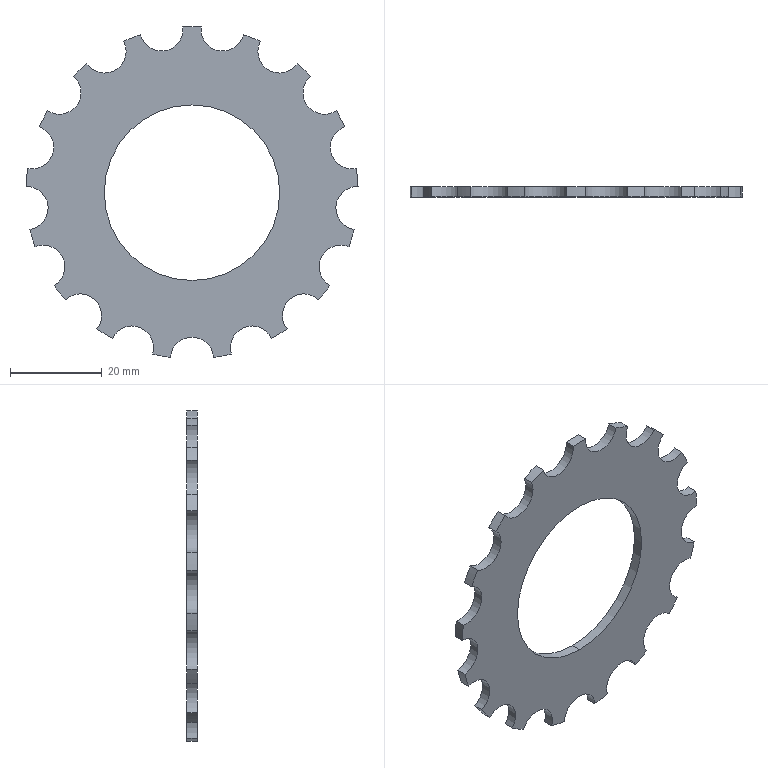Part | STEP file | Gear 4 | 1 solid | 47 faces | box 72.249 x 2.2 x 71.994 mm | volume 5249 mm3 | cylinder 45 | plane 2 | commonest cylinder face diameters 9.4 x26 72.3 x17 38.2 x2